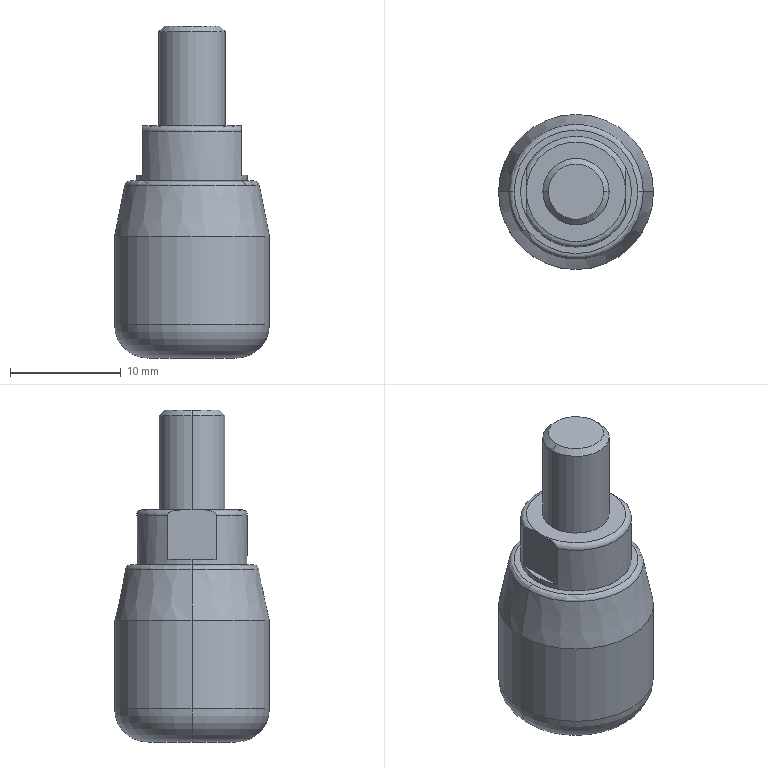Part | SolidWorks | features Fillet 3, ICE 3, Chamfer 2, Extrusion 1 | 1 solid | 24 faces | box 14 x 14 x 30 mm | volume 2911 mm3 | plane 8 | torus 6 | cylinder 6 | cone 4 | commonest cylinder face diameters 6 x2 10 x2 14 x2
STEP:
#1=CARTESIAN_POINT('',(2.5,0.,22.));
#2=VERTEX_POINT('',#1);
#3=CARTESIAN_POINT('',(-2.5,0.,22.));
#4=VERTEX_POINT('',#3);
#5=CARTESIAN_POINT('',(0.,0.,22.));
#6=DIRECTION('',(0.,0.,1.));
#7=DIRECTION('',(1.,0.,0.));
#8=AXIS2_PLACEMENT_3D('',#5,#6,#7);
#9=CIRCLE('',#8,2.5);
#10=EDGE_CURVE('',#2,#4,#9,.T.);
#11=ORIENTED_EDGE('',*,*,#10,.F.);
#12=CARTESIAN_POINT('',(3.,0.,21.5));
#13=VERTEX_POINT('',#12);
#14=CARTESIAN_POINT('',(2.5,0.,22.));
#15=DIRECTION('',(0.7071,0.,-0.7071));
#16=VECTOR('',#15,1000.);
#17=LINE('',#14,#16);
#18=EDGE_CURVE('',#2,#13,#17,.T.);
#19=ORIENTED_EDGE('',*,*,#18,.T.);
#20=CARTESIAN_POINT('',(-3.,0.,21.5));
#21=VERTEX_POINT('',#20);
#22=CARTESIAN_POINT('',(0.,0.,21.5));
#23=DIRECTION('',(0.,0.,-1.));
#24=DIRECTION('',(1.,0.,0.));
#25=AXIS2_PLACEMENT_3D('',#22,#23,#24);
#26=CIRCLE('',#25,3.);
#27=EDGE_CURVE('',#21,#13,#26,.T.);
#28=ORIENTED_EDGE('',*,*,#27,.F.);
#29=CARTESIAN_POINT('',(-2.5,0.,22.));
#30=DIRECTION('',(-0.7071,0.,-0.7071));
#31=VECTOR('',#30,1000.);
#32=LINE('',#29,#31);
#33=EDGE_CURVE('',#4,#21,#32,.T.);
#34=ORIENTED_EDGE('',*,*,#33,.F.);
#35=EDGE_LOOP('',(#11,#19,#28,#34));
#36=FACE_OUTER_BOUND('',#35,.T.);
#37=CARTESIAN_POINT('',(0.,0.,22.));
#38=DIRECTION('',(0.,0.,-1.));
#39=DIRECTION('',(-1.,0.,0.));
#40=AXIS2_PLACEMENT_3D('',#37,#38,#39);
#41=CONICAL_SURFACE('',#40,2.5,0.7854);
#42=ADVANCED_FACE('',(#36),#41,.T.);
#43=CARTESIAN_POINT('',(-6.08,0.,7.598));
#44=VERTEX_POINT('',#43);
#45=CARTESIAN_POINT('',(6.08,0.,7.598));
#46=VERTEX_POINT('',#45);
#47=CARTESIAN_POINT('',(0.,0.,7.598));
#48=DIRECTION('',(0.,0.,-1.));
#49=DIRECTION('',(1.,0.,0.));
#50=AXIS2_PLACEMENT_3D('',#47,#48,#49);
#51=CIRCLE('',#50,6.08);
#52=EDGE_CURVE('',#44,#46,#51,.T.);
#53=ORIENTED_EDGE('',*,*,#52,.F.);
#54=CARTESIAN_POINT('',(-5.59,0.,8.));
#55=VERTEX_POINT('',#54);
#56=CARTESIAN_POINT('',(-5.59,0.,7.5));
#57=DIRECTION('',(0.,1.,0.));
#58=DIRECTION('',(-1.,0.,0.));
#59=AXIS2_PLACEMENT_3D('',#56,#57,#58);
#60=CIRCLE('',#59,0.5);
#61=EDGE_CURVE('',#44,#55,#60,.T.);
#62=ORIENTED_EDGE('',*,*,#61,.T.);
#63=CARTESIAN_POINT('',(5.59,0.,8.));
#64=VERTEX_POINT('',#63);
#65=CARTESIAN_POINT('',(0.,0.,8.));
#66=DIRECTION('',(0.,0.,1.));
#67=DIRECTION('',(1.,0.,0.));
#68=AXIS2_PLACEMENT_3D('',#65,#66,#67);
#69=CIRCLE('',#68,5.59);
#70=EDGE_CURVE('',#64,#55,#69,.T.);
#71=ORIENTED_EDGE('',*,*,#70,.F.);
#72=CARTESIAN_POINT('',(5.59,0.,7.5));
#73=DIRECTION('',(0.,-1.,0.));
#74=DIRECTION('',(0.,0.,-1.));
#75=AXIS2_PLACEMENT_3D('',#72,#73,#74);
#76=CIRCLE('',#75,0.5);
#77=EDGE_CURVE('',#46,#64,#76,.T.);
#78=ORIENTED_EDGE('',*,*,#77,.F.);
#79=EDGE_LOOP('',(#53,#62,#71,#78));
#80=FACE_OUTER_BOUND('',#79,.T.);
#81=CARTESIAN_POINT('',(0.,0.,7.5));
#82=DIRECTION('',(0.,0.,1.));
#83=DIRECTION('',(1.,0.,0.));
#84=AXIS2_PLACEMENT_3D('',#81,#82,#83);
#85=TOROIDAL_SURFACE('',#84,5.59,0.5);
#86=ADVANCED_FACE('',(#80),#85,.T.);
#87=CARTESIAN_POINT('',(-4.,0.,-8.));
#88=VERTEX_POINT('',#87);
#89=CARTESIAN_POINT('',(4.,0.,-8.));
#90=VERTEX_POINT('',#89);
#91=CARTESIAN_POINT('',(0.,0.,-8.));
#92=DIRECTION('',(0.,0.,-1.));
#93=DIRECTION('',(1.,0.,0.));
#94=AXIS2_PLACEMENT_3D('',#91,#92,#93);
#95=CIRCLE('',#94,4.);
#96=EDGE_CURVE('',#88,#90,#95,.T.);
#97=ORIENTED_EDGE('',*,*,#96,.F.);
#98=CARTESIAN_POINT('',(-7.,0.,-5.));
#99=VERTEX_POINT('',#98);
#100=CARTESIAN_POINT('',(-4.,0.,-5.));
#101=DIRECTION('',(0.,1.,0.));
#102=DIRECTION('',(-1.,0.,0.));
#103=AXIS2_PLACEMENT_3D('',#100,#101,#102);
#104=CIRCLE('',#103,3.);
#105=EDGE_CURVE('',#88,#99,#104,.T.);
#106=ORIENTED_EDGE('',*,*,#105,.T.);
#107=CARTESIAN_POINT('',(7.,0.,-5.));
#108=VERTEX_POINT('',#107);
#109=CARTESIAN_POINT('',(0.,0.,-5.));
#110=DIRECTION('',(0.,0.,1.));
#111=DIRECTION('',(1.,0.,0.));
#112=AXIS2_PLACEMENT_3D('',#109,#110,#111);
#113=CIRCLE('',#112,7.);
#114=EDGE_CURVE('',#108,#99,#113,.T.);
#115=ORIENTED_EDGE('',*,*,#114,.F.);
#116=CARTESIAN_POINT('',(4.,0.,-5.));
#117=DIRECTION('',(0.,-1.,0.));
#118=DIRECTION('',(0.,0.,-1.));
#119=AXIS2_PLACEMENT_3D('',#116,#117,#118);
#120=CIRCLE('',#119,3.);
#121=EDGE_CURVE('',#90,#108,#120,.T.);
#122=ORIENTED_EDGE('',*,*,#121,.F.);
#123=EDGE_LOOP('',(#97,#106,#115,#122));
#124=FACE_OUTER_BOUND('',#123,.T.);
#125=CARTESIAN_POINT('',(0.,0.,-5.));
#126=DIRECTION('',(0.,0.,1.));
#127=DIRECTION('',(1.,0.,0.));
#128=AXIS2_PLACEMENT_3D('',#125,#126,#127);
#129=TOROIDAL_SURFACE('',#128,4.,3.);
#130=ADVANCED_FACE('',(#124),#129,.T.);
#131=ORIENTED_EDGE('',*,*,#52,.T.);
#132=CARTESIAN_POINT('',(7.,0.,3.));
#133=VERTEX_POINT('',#132);
#134=CARTESIAN_POINT('',(6.,0.,8.));
#135=DIRECTION('',(0.1961,0.,-0.9806));
#136=VECTOR('',#135,1000.);
#137=LINE('',#134,#136);
#138=EDGE_CURVE('',#46,#133,#137,.T.);
#139=ORIENTED_EDGE('',*,*,#138,.T.);
#140=CARTESIAN_POINT('',(-7.,0.,3.));
#141=VERTEX_POINT('',#140);
#142=CARTESIAN_POINT('',(0.,0.,3.));
#143=DIRECTION('',(0.,0.,-1.));
#144=DIRECTION('',(1.,0.,0.));
#145=AXIS2_PLACEMENT_3D('',#142,#143,#144);
#146=CIRCLE('',#145,7.);
#147=EDGE_CURVE('',#141,#133,#146,.T.);
#148=ORIENTED_EDGE('',*,*,#147,.F.);
#149=CARTESIAN_POINT('',(-6.,0.,8.));
#150=DIRECTION('',(-0.1961,0.,-0.9806));
#151=VECTOR('',#150,1000.);
#152=LINE('',#149,#151);
#153=EDGE_CURVE('',#44,#141,#152,.T.);
#154=ORIENTED_EDGE('',*,*,#153,.F.);
#155=EDGE_LOOP('',(#131,#139,#148,#154));
#156=FACE_OUTER_BOUND('',#155,.T.);
#157=CARTESIAN_POINT('',(0.,0.,8.));
#158=DIRECTION('',(0.,0.,-1.));
#159=DIRECTION('',(-1.,0.,0.));
#160=AXIS2_PLACEMENT_3D('',#157,#158,#159);
#161=CONICAL_SURFACE('',#160,6.,0.1974);
#162=ADVANCED_FACE('',(#156),#161,.T.);
#163=ORIENTED_EDGE('',*,*,#27,.T.);
#164=CARTESIAN_POINT('',(3.,0.,13.));
#165=VERTEX_POINT('',#164);
#166=CARTESIAN_POINT('',(3.,0.,22.));
#167=DIRECTION('',(0.,0.,-1.));
#168=VECTOR('',#167,1000.);
#169=LINE('',#166,#168);
#170=EDGE_CURVE('',#13,#165,#169,.T.);
#171=ORIENTED_EDGE('',*,*,#170,.T.);
#172=CARTESIAN_POINT('',(-3.,0.,13.));
#173=VERTEX_POINT('',#172);
#174=CARTESIAN_POINT('',(0.,0.,13.));
#175=DIRECTION('',(0.,0.,1.));
#176=DIRECTION('',(1.,0.,0.));
#177=AXIS2_PLACEMENT_3D('',#174,#175,#176);
#178=CIRCLE('',#177,3.);
#179=EDGE_CURVE('',#165,#173,#178,.T.);
#180=ORIENTED_EDGE('',*,*,#179,.T.);
#181=CARTESIAN_POINT('',(-3.,0.,22.));
#182=DIRECTION('',(0.,0.,-1.));
#183=VECTOR('',#182,1000.);
#184=LINE('',#181,#183);
#185=EDGE_CURVE('',#21,#173,#184,.T.);
#186=ORIENTED_EDGE('',*,*,#185,.F.);
#187=EDGE_LOOP('',(#163,#171,#180,#186));
#188=FACE_OUTER_BOUND('',#187,.T.);
#189=CARTESIAN_POINT('',(0.,0.,22.));
#190=DIRECTION('',(0.,0.,-1.));
#191=DIRECTION('',(-1.,0.,0.));
#192=AXIS2_PLACEMENT_3D('',#189,#190,#191);
#193=CYLINDRICAL_SURFACE('',#192,3.);
#194=ADVANCED_FACE('',(#188),#193,.T.);
#195=ORIENTED_EDGE('',*,*,#147,.T.);
#196=CARTESIAN_POINT('',(7.,0.,8.));
#197=DIRECTION('',(0.,0.,-1.));
#198=VECTOR('',#197,1000.);
#199=LINE('',#196,#198);
#200=EDGE_CURVE('',#133,#108,#199,.T.);
#201=ORIENTED_EDGE('',*,*,#200,.T.);
#202=ORIENTED_EDGE('',*,*,#114,.T.);
#203=CARTESIAN_POINT('',(-7.,0.,8.));
#204=DIRECTION('',(0.,0.,-1.));
#205=VECTOR('',#204,1000.);
#206=LINE('',#203,#205);
#207=EDGE_CURVE('',#141,#99,#206,.T.);
#208=ORIENTED_EDGE('',*,*,#207,.F.);
#209=EDGE_LOOP('',(#195,#201,#202,#208));
#210=FACE_OUTER_BOUND('',#209,.T.);
#211=CARTESIAN_POINT('',(0.,0.,8.));
#212=DIRECTION('',(0.,0.,-1.));
#213=DIRECTION('',(-1.,0.,0.));
#214=AXIS2_PLACEMENT_3D('',#211,#212,#213);
#215=CYLINDRICAL_SURFACE('',#214,7.);
#216=ADVANCED_FACE('',(#210),#215,.T.);
#217=CARTESIAN_POINT('',(5.,0.,8.5));
#218=VERTEX_POINT('',#217);
#219=CARTESIAN_POINT('',(4.5,2.179,8.5));
#220=VERTEX_POINT('',#219);
#221=CARTESIAN_POINT('',(0.,0.,8.5));
#222=DIRECTION('',(0.,0.,1.));
#223=DIRECTION('',(1.,0.,0.));
#224=AXIS2_PLACEMENT_3D('',#221,#222,#223);
#225=CIRCLE('',#224,5.);
#226=EDGE_CURVE('',#218,#220,#225,.T.);
#227=ORIENTED_EDGE('',*,*,#226,.F.);
#228=CARTESIAN_POINT('',(5.,0.,8.));
#229=VERTEX_POINT('',#228);
#230=CARTESIAN_POINT('',(5.,0.,13.));
#231=DIRECTION('',(0.,0.,-1.));
#232=VECTOR('',#231,1000.);
#233=LINE('',#230,#232);
#234=EDGE_CURVE('',#218,#229,#233,.T.);
#235=ORIENTED_EDGE('',*,*,#234,.T.);
#236=CARTESIAN_POINT('',(-5.,0.,8.));
#237=VERTEX_POINT('',#236);
#238=CARTESIAN_POINT('',(0.,0.,8.));
#239=DIRECTION('',(0.,0.,1.));
#240=DIRECTION('',(1.,0.,0.));
#241=AXIS2_PLACEMENT_3D('',#238,#239,#240);
#242=CIRCLE('',#241,5.);
#243=EDGE_CURVE('',#229,#237,#242,.T.);
#244=ORIENTED_EDGE('',*,*,#243,.T.);
#245=CARTESIAN_POINT('',(-5.,0.,8.5));
#246=VERTEX_POINT('',#245);
#247=CARTESIAN_POINT('',(-5.,0.,13.));
#248=DIRECTION('',(0.,0.,-1.));
#249=VECTOR('',#248,1000.);
#250=LINE('',#247,#249);
#251=EDGE_CURVE('',#246,#237,#250,.T.);
#252=ORIENTED_EDGE('',*,*,#251,.F.);
#253=CARTESIAN_POINT('',(-4.5,2.179,8.5));
#254=VERTEX_POINT('',#253);
#255=CARTESIAN_POINT('',(0.,0.,8.5));
#256=DIRECTION('',(0.,0.,1.));
#257=DIRECTION('',(1.,0.,0.));
#258=AXIS2_PLACEMENT_3D('',#255,#256,#257);
#259=CIRCLE('',#258,5.);
#260=EDGE_CURVE('',#254,#246,#259,.T.);
#261=ORIENTED_EDGE('',*,*,#260,.F.);
#262=CARTESIAN_POINT('',(-4.5,2.179,12.5));
#263=VERTEX_POINT('',#262);
#264=CARTESIAN_POINT('',(-4.5,2.179,13.));
#265=DIRECTION('',(0.,0.,-1.));
#266=VECTOR('',#265,1000.);
#267=LINE('',#264,#266);
#268=EDGE_CURVE('',#263,#254,#267,.T.);
#269=ORIENTED_EDGE('',*,*,#268,.F.);
#270=CARTESIAN_POINT('',(4.5,2.179,12.5));
#271=VERTEX_POINT('',#270);
#272=CARTESIAN_POINT('',(0.,0.,12.5));
#273=DIRECTION('',(0.,0.,-1.));
#274=DIRECTION('',(1.,0.,0.));
#275=AXIS2_PLACEMENT_3D('',#272,#273,#274);
#276=CIRCLE('',#275,5.);
#277=EDGE_CURVE('',#263,#271,#276,.T.);
#278=ORIENTED_EDGE('',*,*,#277,.T.);
#279=CARTESIAN_POINT('',(4.5,2.179,13.));
#280=DIRECTION('',(0.,0.,1.));
#281=VECTOR('',#280,1000.);
#282=LINE('',#279,#281);
#283=EDGE_CURVE('',#220,#271,#282,.T.);
#284=ORIENTED_EDGE('',*,*,#283,.F.);
#285=EDGE_LOOP('',(#227,#235,#244,#252,#261,#269,#278,#284));
#286=FACE_OUTER_BOUND('',#285,.T.);
#287=CARTESIAN_POINT('',(0.,0.,13.));
#288=DIRECTION('',(0.,0.,-1.));
#289=DIRECTION('',(-1.,0.,0.));
#290=AXIS2_PLACEMENT_3D('',#287,#288,#289);
#291=CYLINDRICAL_SURFACE('',#290,5.);
#292=ADVANCED_FACE('',(#286),#291,.T.);
#293=ORIENTED_EDGE('',*,*,#234,.F.);
#294=CARTESIAN_POINT('',(4.5,-2.179,8.5));
#295=VERTEX_POINT('',#294);
#296=CARTESIAN_POINT('',(0.,0.,8.5));
#297=DIRECTION('',(0.,0.,1.));
#298=DIRECTION('',(1.,0.,0.));
#299=AXIS2_PLACEMENT_3D('',#296,#297,#298);
#300=CIRCLE('',#299,5.);
#301=EDGE_CURVE('',#295,#218,#300,.T.);
#302=ORIENTED_EDGE('',*,*,#301,.F.);
#303=CARTESIAN_POINT('',(4.5,-2.179,12.5));
#304=VERTEX_POINT('',#303);
#305=CARTESIAN_POINT('',(4.5,-2.179,13.));
#306=DIRECTION('',(0.,0.,-1.));
#307=VECTOR('',#306,1000.);
#308=LINE('',#305,#307);
#309=EDGE_CURVE('',#304,#295,#308,.T.);
#310=ORIENTED_EDGE('',*,*,#309,.F.);
#311=CARTESIAN_POINT('',(-4.5,-2.179,12.5));
#312=VERTEX_POINT('',#311);
#313=CARTESIAN_POINT('',(0.,0.,12.5));
#314=DIRECTION('',(0.,0.,-1.));
#315=DIRECTION('',(1.,0.,0.));
#316=AXIS2_PLACEMENT_3D('',#313,#314,#315);
#317=CIRCLE('',#316,5.);
#318=EDGE_CURVE('',#304,#312,#317,.T.);
#319=ORIENTED_EDGE('',*,*,#318,.T.);
#320=CARTESIAN_POINT('',(-4.5,-2.179,8.5));
#321=VERTEX_POINT('',#320);
#322=CARTESIAN_POINT('',(-4.5,-2.179,13.));
#323=DIRECTION('',(0.,0.,1.));
#324=VECTOR('',#323,1000.);
#325=LINE('',#322,#324);
#326=EDGE_CURVE('',#321,#312,#325,.T.);
#327=ORIENTED_EDGE('',*,*,#326,.F.);
#328=CARTESIAN_POINT('',(0.,0.,8.5));
#329=DIRECTION('',(0.,0.,1.));
#330=DIRECTION('',(1.,0.,0.));
#331=AXIS2_PLACEMENT_3D('',#328,#329,#330);
#332=CIRCLE('',#331,5.);
#333=EDGE_CURVE('',#246,#321,#332,.T.);
#334=ORIENTED_EDGE('',*,*,#333,.F.);
#335=ORIENTED_EDGE('',*,*,#251,.T.);
#336=CARTESIAN_POINT('',(0.,0.,8.));
#337=DIRECTION('',(0.,0.,1.));
#338=DIRECTION('',(1.,0.,0.));
#339=AXIS2_PLACEMENT_3D('',#336,#337,#338);
#340=CIRCLE('',#339,5.);
#341=EDGE_CURVE('',#237,#229,#340,.T.);
#342=ORIENTED_EDGE('',*,*,#341,.T.);
#343=EDGE_LOOP('',(#293,#302,#310,#319,#327,#334,#335,#342));
#344=FACE_OUTER_BOUND('',#343,.T.);
#345=CARTESIAN_POINT('',(0.,0.,13.));
#346=DIRECTION('',(0.,0.,-1.));
#347=DIRECTION('',(-1.,0.,0.));
#348=AXIS2_PLACEMENT_3D('',#345,#346,#347);
#349=CYLINDRICAL_SURFACE('',#348,5.);
#350=ADVANCED_FACE('',(#344),#349,.T.);
#351=CARTESIAN_POINT('',(4.5,0.,13.));
#352=VERTEX_POINT('',#351);
#353=CARTESIAN_POINT('',(-4.5,0.,13.));
#354=VERTEX_POINT('',#353);
#355=CARTESIAN_POINT('',(0.,0.,13.));
#356=DIRECTION('',(0.,0.,1.));
#357=DIRECTION('',(1.,0.,0.));
#358=AXIS2_PLACEMENT_3D('',#355,#356,#357);
#359=CIRCLE('',#358,4.5);
#360=EDGE_CURVE('',#352,#354,#359,.T.);
#361=ORIENTED_EDGE('',*,*,#360,.F.);
#362=CARTESIAN_POINT('',(4.5,0.,13.));
#363=CARTESIAN_POINT('',(4.5,0.1972,13.));
#364=CARTESIAN_POINT('',(4.5,0.3943,13.));
#365=CARTESIAN_POINT('',(4.5,0.7886,12.997));
#366=CARTESIAN_POINT('',(4.5,0.9861,12.992));
#367=CARTESIAN_POINT('',(4.5,1.379,12.96));
#368=CARTESIAN_POINT('',(4.5,1.576,12.934));
#369=CARTESIAN_POINT('',(4.5,1.857,12.842));
#370=CARTESIAN_POINT('',(4.5,1.948,12.803));
#371=CARTESIAN_POINT('',(4.5,2.069,12.715));
#372=CARTESIAN_POINT('',(4.5,2.106,12.681));
#373=CARTESIAN_POINT('',(4.5,2.161,12.599));
#374=CARTESIAN_POINT('',(4.5,2.179,12.549));
#375=CARTESIAN_POINT('',(4.5,2.179,12.5));
#376=B_SPLINE_CURVE_WITH_KNOTS('',3,(#362,#363,#364,#365,#366,#367,#368,#369,#370,#371,#372,#373,#374,#375),.UNSPECIFIED.,.F.,.F.,(4,2,2,2,2,2,4),(0.,0.0005914,0.001183,0.001774,0.00207,0.002218,0.002366),.UNSPECIFIED.);
#377=EDGE_CURVE('',#352,#271,#376,.T.);
#378=ORIENTED_EDGE('',*,*,#377,.T.);
#379=ORIENTED_EDGE('',*,*,#277,.F.);
#380=CARTESIAN_POINT('',(-4.5,2.179,12.5));
#381=CARTESIAN_POINT('',(-4.5,2.179,12.55));
#382=CARTESIAN_POINT('',(-4.5,2.161,12.599));
#383=CARTESIAN_POINT('',(-4.5,2.105,12.681));
#384=CARTESIAN_POINT('',(-4.5,2.068,12.716));
#385=CARTESIAN_POINT('',(-4.5,1.948,12.804));
#386=CARTESIAN_POINT('',(-4.5,1.855,12.843));
#387=CARTESIAN_POINT('',(-4.5,1.574,12.934));
#388=CARTESIAN_POINT('',(-4.5,1.377,12.96));
#389=CARTESIAN_POINT('',(-4.5,0.9842,12.992));
#390=CARTESIAN_POINT('',(-4.5,0.7874,12.997));
#391=CARTESIAN_POINT('',(-4.5,0.3938,13.));
#392=CARTESIAN_POINT('',(-4.5,0.1985,13.));
#393=CARTESIAN_POINT('',(-4.5,0.,13.));
#394=B_SPLINE_CURVE_WITH_KNOTS('',3,(#380,#381,#382,#383,#384,#385,#386,#387,#388,#389,#390,#391,#392,#393),.UNSPECIFIED.,.F.,.F.,(4,2,2,2,2,2,4),(0.007127,0.007276,0.007425,0.007723,0.008318,0.008913,0.009509),.UNSPECIFIED.);
#395=EDGE_CURVE('',#263,#354,#394,.T.);
#396=ORIENTED_EDGE('',*,*,#395,.T.);
#397=EDGE_LOOP('',(#361,#378,#379,#396));
#398=FACE_OUTER_BOUND('',#397,.T.);
#399=CARTESIAN_POINT('',(0.,0.,12.5));
#400=DIRECTION('',(0.,0.,1.));
#401=DIRECTION('',(1.,0.,0.));
#402=AXIS2_PLACEMENT_3D('',#399,#400,#401);
#403=TOROIDAL_SURFACE('',#402,4.5,0.5);
#404=ADVANCED_FACE('',(#398),#403,.T.);
#405=ORIENTED_EDGE('',*,*,#318,.F.);
#406=CARTESIAN_POINT('',(4.5,-2.179,12.5));
#407=CARTESIAN_POINT('',(4.5,-2.179,12.55));
#408=CARTESIAN_POINT('',(4.5,-2.161,12.599));
#409=CARTESIAN_POINT('',(4.5,-2.105,12.681));
#410=CARTESIAN_POINT('',(4.5,-2.068,12.716));
#411=CARTESIAN_POINT('',(4.5,-1.948,12.804));
#412=CARTESIAN_POINT('',(4.5,-1.855,12.843));
#413=CARTESIAN_POINT('',(4.5,-1.574,12.934));
#414=CARTESIAN_POINT('',(4.5,-1.377,12.96));
#415=CARTESIAN_POINT('',(4.5,-0.9842,12.992));
#416=CARTESIAN_POINT('',(4.5,-0.7874,12.997));
#417=CARTESIAN_POINT('',(4.5,-0.3938,13.));
#418=CARTESIAN_POINT('',(4.5,-0.1985,13.));
#419=CARTESIAN_POINT('',(4.5,0.,13.));
#420=B_SPLINE_CURVE_WITH_KNOTS('',3,(#406,#407,#408,#409,#410,#411,#412,#413,#414,#415,#416,#417,#418,#419),.UNSPECIFIED.,.F.,.F.,(4,2,2,2,2,2,4),(0.007127,0.007276,0.007425,0.007723,0.008318,0.008913,0.009509),.UNSPECIFIED.);
#421=EDGE_CURVE('',#304,#352,#420,.T.);
#422=ORIENTED_EDGE('',*,*,#421,.T.);
#423=CARTESIAN_POINT('',(0.,0.,13.));
#424=DIRECTION('',(0.,0.,1.));
#425=DIRECTION('',(1.,0.,0.));
#426=AXIS2_PLACEMENT_3D('',#423,#424,#425);
#427=CIRCLE('',#426,4.5);
#428=EDGE_CURVE('',#354,#352,#427,.T.);
#429=ORIENTED_EDGE('',*,*,#428,.F.);
#430=CARTESIAN_POINT('',(-4.5,0.,13.));
#431=CARTESIAN_POINT('',(-4.5,-0.1972,13.));
#432=CARTESIAN_POINT('',(-4.5,-0.3943,13.));
#433=CARTESIAN_POINT('',(-4.5,-0.7886,12.997));
#434=CARTESIAN_POINT('',(-4.5,-0.9861,12.992));
#435=CARTESIAN_POINT('',(-4.5,-1.379,12.96));
#436=CARTESIAN_POINT('',(-4.5,-1.576,12.934));
#437=CARTESIAN_POINT('',(-4.5,-1.857,12.842));
#438=CARTESIAN_POINT('',(-4.5,-1.948,12.803));
#439=CARTESIAN_POINT('',(-4.5,-2.069,12.715));
#440=CARTESIAN_POINT('',(-4.5,-2.106,12.681));
#441=CARTESIAN_POINT('',(-4.5,-2.161,12.599));
#442=CARTESIAN_POINT('',(-4.5,-2.179,12.549));
#443=CARTESIAN_POINT('',(-4.5,-2.179,12.5));
#444=B_SPLINE_CURVE_WITH_KNOTS('',3,(#430,#431,#432,#433,#434,#435,#436,#437,#438,#439,#440,#441,#442,#443),.UNSPECIFIED.,.F.,.F.,(4,2,2,2,2,2,4),(0.,0.0005914,0.001183,0.001774,0.00207,0.002218,0.002366),.UNSPECIFIED.);
#445=EDGE_CURVE('',#354,#312,#444,.T.);
#446=ORIENTED_EDGE('',*,*,#445,.T.);
#447=EDGE_LOOP('',(#405,#422,#429,#446));
#448=FACE_OUTER_BOUND('',#447,.T.);
#449=CARTESIAN_POINT('',(0.,0.,12.5));
#450=DIRECTION('',(0.,0.,1.));
#451=DIRECTION('',(1.,0.,0.));
#452=AXIS2_PLACEMENT_3D('',#449,#450,#451);
#453=TOROIDAL_SURFACE('',#452,4.5,0.5);
#454=ADVANCED_FACE('',(#448),#453,.T.);
#455=ORIENTED_EDGE('',*,*,#360,.T.);
#456=ORIENTED_EDGE('',*,*,#428,.T.);
#457=EDGE_LOOP('',(#455,#456));
#458=FACE_OUTER_BOUND('',#457,.T.);
#459=CARTESIAN_POINT('',(0.,0.,13.));
#460=DIRECTION('',(0.,0.,1.));
#461=DIRECTION('',(1.,0.,0.));
#462=AXIS2_PLACEMENT_3D('',#459,#460,#461);
#463=CIRCLE('',#462,3.);
#464=EDGE_CURVE('',#173,#165,#463,.T.);
#465=ORIENTED_EDGE('',*,*,#464,.F.);
#466=ORIENTED_EDGE('',*,*,#179,.F.);
#467=EDGE_LOOP('',(#465,#466));
#468=FACE_BOUND('',#467,.T.);
#469=CARTESIAN_POINT('',(0.,0.,13.));
#470=DIRECTION('',(0.,0.,1.));
#471=DIRECTION('',(1.,0.,0.));
#472=AXIS2_PLACEMENT_3D('',#469,#470,#471);
#473=PLANE('',#472);
#474=ADVANCED_FACE('',(#458,#468),#473,.T.);
#475=ORIENTED_EDGE('',*,*,#70,.T.);
#476=CARTESIAN_POINT('',(0.,0.,8.));
#477=DIRECTION('',(0.,0.,1.));
#478=DIRECTION('',(1.,0.,0.));
#479=AXIS2_PLACEMENT_3D('',#476,#477,#478);
#480=CIRCLE('',#479,5.59);
#481=EDGE_CURVE('',#55,#64,#480,.T.);
#482=ORIENTED_EDGE('',*,*,#481,.T.);
#483=EDGE_LOOP('',(#475,#482));
#484=FACE_OUTER_BOUND('',#483,.T.);
#485=ORIENTED_EDGE('',*,*,#341,.F.);
#486=ORIENTED_EDGE('',*,*,#243,.F.);
#487=EDGE_LOOP('',(#485,#486));
#488=FACE_BOUND('',#487,.T.);
#489=CARTESIAN_POINT('',(0.,0.,8.));
#490=DIRECTION('',(0.,0.,1.));
#491=DIRECTION('',(1.,0.,0.));
#492=AXIS2_PLACEMENT_3D('',#489,#490,#491);
#493=PLANE('',#492);
#494=ADVANCED_FACE('',(#484,#488),#493,.T.);
#495=ORIENTED_EDGE('',*,*,#200,.F.);
#496=CARTESIAN_POINT('',(0.,0.,3.));
#497=DIRECTION('',(0.,0.,-1.));
#498=DIRECTION('',(1.,0.,0.));
#499=AXIS2_PLACEMENT_3D('',#496,#497,#498);
#500=CIRCLE('',#499,7.);
#501=EDGE_CURVE('',#133,#141,#500,.T.);
#502=ORIENTED_EDGE('',*,*,#501,.T.);
#503=ORIENTED_EDGE('',*,*,#207,.T.);
#504=CARTESIAN_POINT('',(0.,0.,-5.));
#505=DIRECTION('',(0.,0.,1.));
#506=DIRECTION('',(1.,0.,0.));
#507=AXIS2_PLACEMENT_3D('',#504,#505,#506);
#508=CIRCLE('',#507,7.);
#509=EDGE_CURVE('',#99,#108,#508,.T.);
#510=ORIENTED_EDGE('',*,*,#509,.T.);
#511=EDGE_LOOP('',(#495,#502,#503,#510));
#512=FACE_OUTER_BOUND('',#511,.T.);
#513=CARTESIAN_POINT('',(0.,0.,8.));
#514=DIRECTION('',(0.,0.,-1.));
#515=DIRECTION('',(-1.,0.,0.));
#516=AXIS2_PLACEMENT_3D('',#513,#514,#515);
#517=CYLINDRICAL_SURFACE('',#516,7.);
#518=ADVANCED_FACE('',(#512),#517,.T.);
#519=CARTESIAN_POINT('',(0.,0.,-8.));
#520=DIRECTION('',(0.,0.,-1.));
#521=DIRECTION('',(1.,0.,0.));
#522=AXIS2_PLACEMENT_3D('',#519,#520,#521);
#523=CIRCLE('',#522,4.);
#524=EDGE_CURVE('',#90,#88,#523,.T.);
#525=ORIENTED_EDGE('',*,*,#524,.T.);
#526=ORIENTED_EDGE('',*,*,#96,.T.);
#527=EDGE_LOOP('',(#525,#526));
#528=FACE_OUTER_BOUND('',#527,.T.);
#529=CARTESIAN_POINT('',(0.,0.,-8.));
#530=DIRECTION('',(0.,0.,1.));
#531=DIRECTION('',(1.,0.,0.));
#532=AXIS2_PLACEMENT_3D('',#529,#530,#531);
#533=PLANE('',#532);
#534=ADVANCED_FACE('',(#528),#533,.F.);
#535=ORIENTED_EDGE('',*,*,#170,.F.);
#536=CARTESIAN_POINT('',(0.,0.,21.5));
#537=DIRECTION('',(0.,0.,-1.));
#538=DIRECTION('',(1.,0.,0.));
#539=AXIS2_PLACEMENT_3D('',#536,#537,#538);
#540=CIRCLE('',#539,3.);
#541=EDGE_CURVE('',#13,#21,#540,.T.);
#542=ORIENTED_EDGE('',*,*,#541,.T.);
#543=ORIENTED_EDGE('',*,*,#185,.T.);
#544=ORIENTED_EDGE('',*,*,#464,.T.);
#545=EDGE_LOOP('',(#535,#542,#543,#544));
#546=FACE_OUTER_BOUND('',#545,.T.);
#547=CARTESIAN_POINT('',(0.,0.,22.));
#548=DIRECTION('',(0.,0.,-1.));
#549=DIRECTION('',(-1.,0.,0.));
#550=AXIS2_PLACEMENT_3D('',#547,#548,#549);
#551=CYLINDRICAL_SURFACE('',#550,3.);
#552=ADVANCED_FACE('',(#546),#551,.T.);
#553=CARTESIAN_POINT('',(0.,0.,22.));
#554=DIRECTION('',(0.,0.,1.));
#555=DIRECTION('',(1.,0.,0.));
#556=AXIS2_PLACEMENT_3D('',#553,#554,#555);
#557=CIRCLE('',#556,2.5);
#558=EDGE_CURVE('',#4,#2,#557,.T.);
#559=ORIENTED_EDGE('',*,*,#558,.T.);
#560=ORIENTED_EDGE('',*,*,#10,.T.);
#561=EDGE_LOOP('',(#559,#560));
#562=FACE_OUTER_BOUND('',#561,.T.);
#563=CARTESIAN_POINT('',(0.,0.,22.));
#564=DIRECTION('',(0.,0.,1.));
#565=DIRECTION('',(1.,0.,0.));
#566=AXIS2_PLACEMENT_3D('',#563,#564,#565);
#567=PLANE('',#566);
#568=ADVANCED_FACE('',(#562),#567,.T.);
#569=ORIENTED_EDGE('',*,*,#138,.F.);
#570=CARTESIAN_POINT('',(0.,0.,7.598));
#571=DIRECTION('',(0.,0.,-1.));
#572=DIRECTION('',(1.,0.,0.));
#573=AXIS2_PLACEMENT_3D('',#570,#571,#572);
#574=CIRCLE('',#573,6.08);
#575=EDGE_CURVE('',#46,#44,#574,.T.);
#576=ORIENTED_EDGE('',*,*,#575,.T.);
#577=ORIENTED_EDGE('',*,*,#153,.T.);
#578=ORIENTED_EDGE('',*,*,#501,.F.);
#579=EDGE_LOOP('',(#569,#576,#577,#578));
#580=FACE_OUTER_BOUND('',#579,.T.);
#581=CARTESIAN_POINT('',(0.,0.,8.));
#582=DIRECTION('',(0.,0.,-1.));
#583=DIRECTION('',(-1.,0.,0.));
#584=AXIS2_PLACEMENT_3D('',#581,#582,#583);
#585=CONICAL_SURFACE('',#584,6.,0.1974);
#586=ADVANCED_FACE('',(#580),#585,.T.);
#587=ORIENTED_EDGE('',*,*,#105,.F.);
#588=ORIENTED_EDGE('',*,*,#524,.F.);
#589=ORIENTED_EDGE('',*,*,#121,.T.);
#590=ORIENTED_EDGE('',*,*,#509,.F.);
#591=EDGE_LOOP('',(#587,#588,#589,#590));
#592=FACE_OUTER_BOUND('',#591,.T.);
#593=CARTESIAN_POINT('',(0.,0.,-5.));
#594=DIRECTION('',(0.,0.,1.));
#595=DIRECTION('',(1.,0.,0.));
#596=AXIS2_PLACEMENT_3D('',#593,#594,#595);
#597=TOROIDAL_SURFACE('',#596,4.,3.);
#598=ADVANCED_FACE('',(#592),#597,.T.);
#599=ORIENTED_EDGE('',*,*,#61,.F.);
#600=ORIENTED_EDGE('',*,*,#575,.F.);
#601=ORIENTED_EDGE('',*,*,#77,.T.);
#602=ORIENTED_EDGE('',*,*,#481,.F.);
#603=EDGE_LOOP('',(#599,#600,#601,#602));
#604=FACE_OUTER_BOUND('',#603,.T.);
#605=CARTESIAN_POINT('',(0.,0.,7.5));
#606=DIRECTION('',(0.,0.,1.));
#607=DIRECTION('',(1.,0.,0.));
#608=AXIS2_PLACEMENT_3D('',#605,#606,#607);
#609=TOROIDAL_SURFACE('',#608,5.59,0.5);
#610=ADVANCED_FACE('',(#604),#609,.T.);
#611=ORIENTED_EDGE('',*,*,#268,.T.);
#612=CARTESIAN_POINT('',(-4.5,5.,8.5));
#613=DIRECTION('',(0.,-1.,0.));
#614=VECTOR('',#613,1000.);
#615=LINE('',#612,#614);
#616=EDGE_CURVE('',#254,#321,#615,.T.);
#617=ORIENTED_EDGE('',*,*,#616,.T.);
#618=ORIENTED_EDGE('',*,*,#326,.T.);
#619=ORIENTED_EDGE('',*,*,#445,.F.);
#620=ORIENTED_EDGE('',*,*,#395,.F.);
#621=EDGE_LOOP('',(#611,#617,#618,#619,#620));
#622=FACE_OUTER_BOUND('',#621,.T.);
#623=CARTESIAN_POINT('',(-4.5,5.,8.5));
#624=DIRECTION('',(-1.,0.,0.));
#625=DIRECTION('',(0.,-1.,0.));
#626=AXIS2_PLACEMENT_3D('',#623,#624,#625);
#627=PLANE('',#626);
#628=ADVANCED_FACE('',(#622),#627,.T.);
#629=ORIENTED_EDGE('',*,*,#260,.T.);
#630=ORIENTED_EDGE('',*,*,#333,.T.);
#631=ORIENTED_EDGE('',*,*,#616,.F.);
#632=EDGE_LOOP('',(#629,#630,#631));
#633=FACE_OUTER_BOUND('',#632,.T.);
#634=CARTESIAN_POINT('',(0.,0.,8.5));
#635=DIRECTION('',(0.,0.,1.));
#636=DIRECTION('',(1.,0.,0.));
#637=AXIS2_PLACEMENT_3D('',#634,#635,#636);
#638=PLANE('',#637);
#639=ADVANCED_FACE('',(#633),#638,.T.);
#640=ORIENTED_EDGE('',*,*,#301,.T.);
#641=ORIENTED_EDGE('',*,*,#226,.T.);
#642=CARTESIAN_POINT('',(4.5,5.,8.5));
#643=DIRECTION('',(0.,1.,0.));
#644=VECTOR('',#643,1000.);
#645=LINE('',#642,#644);
#646=EDGE_CURVE('',#295,#220,#645,.T.);
#647=ORIENTED_EDGE('',*,*,#646,.F.);
#648=EDGE_LOOP('',(#640,#641,#647));
#649=FACE_OUTER_BOUND('',#648,.T.);
#650=CARTESIAN_POINT('',(0.,0.,8.5));
#651=DIRECTION('',(0.,0.,1.));
#652=DIRECTION('',(1.,0.,0.));
#653=AXIS2_PLACEMENT_3D('',#650,#651,#652);
#654=PLANE('',#653);
#655=ADVANCED_FACE('',(#649),#654,.T.);
#656=ORIENTED_EDGE('',*,*,#309,.T.);
#657=ORIENTED_EDGE('',*,*,#646,.T.);
#658=ORIENTED_EDGE('',*,*,#283,.T.);
#659=ORIENTED_EDGE('',*,*,#377,.F.);
#660=ORIENTED_EDGE('',*,*,#421,.F.);
#661=EDGE_LOOP('',(#656,#657,#658,#659,#660));
#662=FACE_OUTER_BOUND('',#661,.T.);
#663=CARTESIAN_POINT('',(4.5,5.,8.5));
#664=DIRECTION('',(1.,0.,0.));
#665=DIRECTION('',(0.,1.,0.));
#666=AXIS2_PLACEMENT_3D('',#663,#664,#665);
#667=PLANE('',#666);
#668=ADVANCED_FACE('',(#662),#667,.T.);
#669=ORIENTED_EDGE('',*,*,#18,.F.);
#670=ORIENTED_EDGE('',*,*,#558,.F.);
#671=ORIENTED_EDGE('',*,*,#33,.T.);
#672=ORIENTED_EDGE('',*,*,#541,.F.);
#673=EDGE_LOOP('',(#669,#670,#671,#672));
#674=FACE_OUTER_BOUND('',#673,.T.);
#675=CARTESIAN_POINT('',(0.,0.,22.));
#676=DIRECTION('',(0.,0.,-1.));
#677=DIRECTION('',(-1.,0.,0.));
#678=AXIS2_PLACEMENT_3D('',#675,#676,#677);
#679=CONICAL_SURFACE('',#678,2.5,0.7854);
#680=ADVANCED_FACE('',(#674),#679,.T.);
#681=CLOSED_SHELL('',(#42,#86,#130,#162,#194,#216,#292,#350,#404,#454,#474,#494,#518,#534,#552,#568,#586,#598,#610,#628,#639,#655,#668,#680));
#682=MANIFOLD_SOLID_BREP('',#681);
#683=CARTESIAN_POINT('',(0.,0.,0.));
#684=DIRECTION('',(0.,0.,1.));
#685=DIRECTION('',(1.,0.,0.));
#686=AXIS2_PLACEMENT_3D('',#683,#684,#685);
#687=(LENGTH_UNIT()NAMED_UNIT(*)SI_UNIT(.MILLI.,.METRE.));
#688=UNCERTAINTY_MEASURE_WITH_UNIT(LENGTH_MEASURE(0.00001),#687,'','');
#689=(NAMED_UNIT(*)PLANE_ANGLE_UNIT()SI_UNIT($,.RADIAN.));
#690=(NAMED_UNIT(*)SI_UNIT($,.STERADIAN.)SOLID_ANGLE_UNIT());
#691=(GEOMETRIC_REPRESENTATION_CONTEXT(3)GLOBAL_UNCERTAINTY_ASSIGNED_CONTEXT((#688))GLOBAL_UNIT_ASSIGNED_CONTEXT((#687,#689,#690))REPRESENTATION_CONTEXT('',''));
#692=ADVANCED_BREP_SHAPE_REPRESENTATION('',(#682,#686),#691);